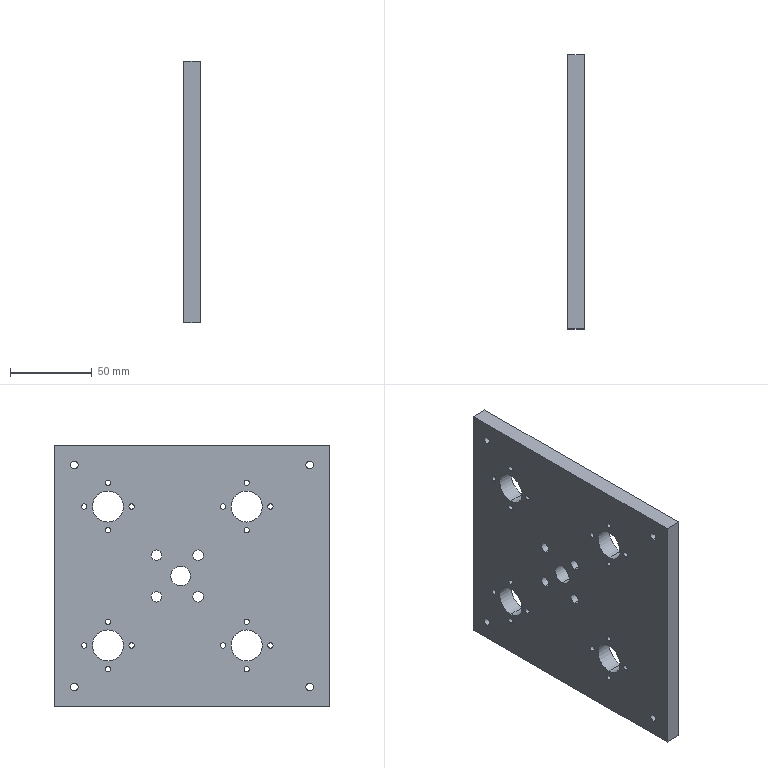Part | STEP file | 03-15 Suction column cylinder fixing plate | 1 solid | 76 faces | box 10 x 168 x 160 mm | volume 252042 mm3 | cylinder 66 | plane 10 | commonest cylinder face diameters 3.3 x32 4.5 x8 6.5 x8 9 x8 19 x8 12 x2